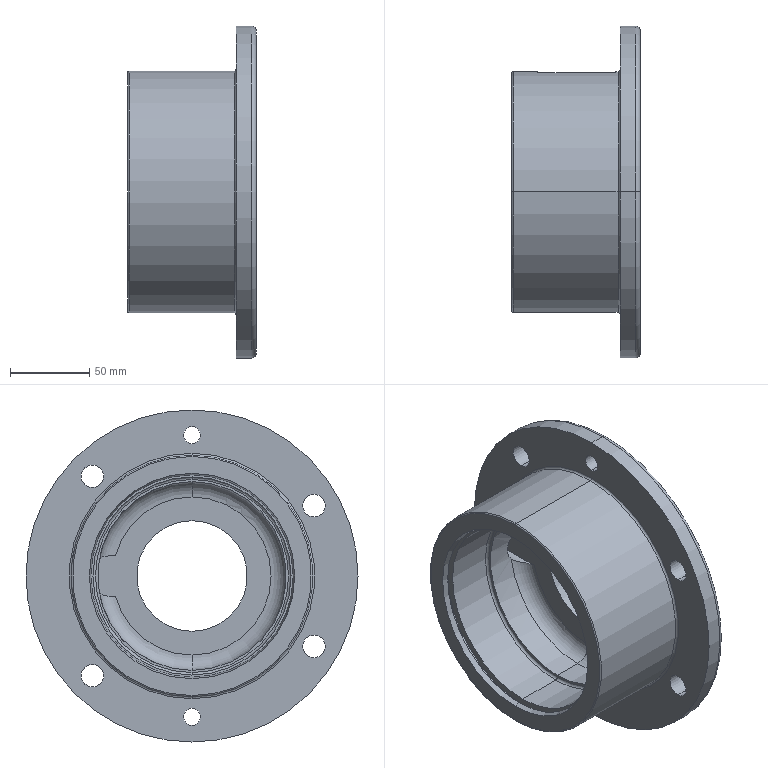Part | SolidWorks | features Fillet 5, ICE 5, Chamfer 2, HoleWzd 2, 3DProfileFeature 1, MirrorPattern 1, Revolution 1 | 1 solid | 190 faces | box 80.975 x 209.55 x 209.55 mm | volume 817016 mm3 | plane 102 | spline 42 | cylinder 29 | torus 13 | cone 4 | commonest cylinder face diameters 14.287 x8 10.716 x4 6.096 x2 69.85 x2 82.55 x2 119.126 x2